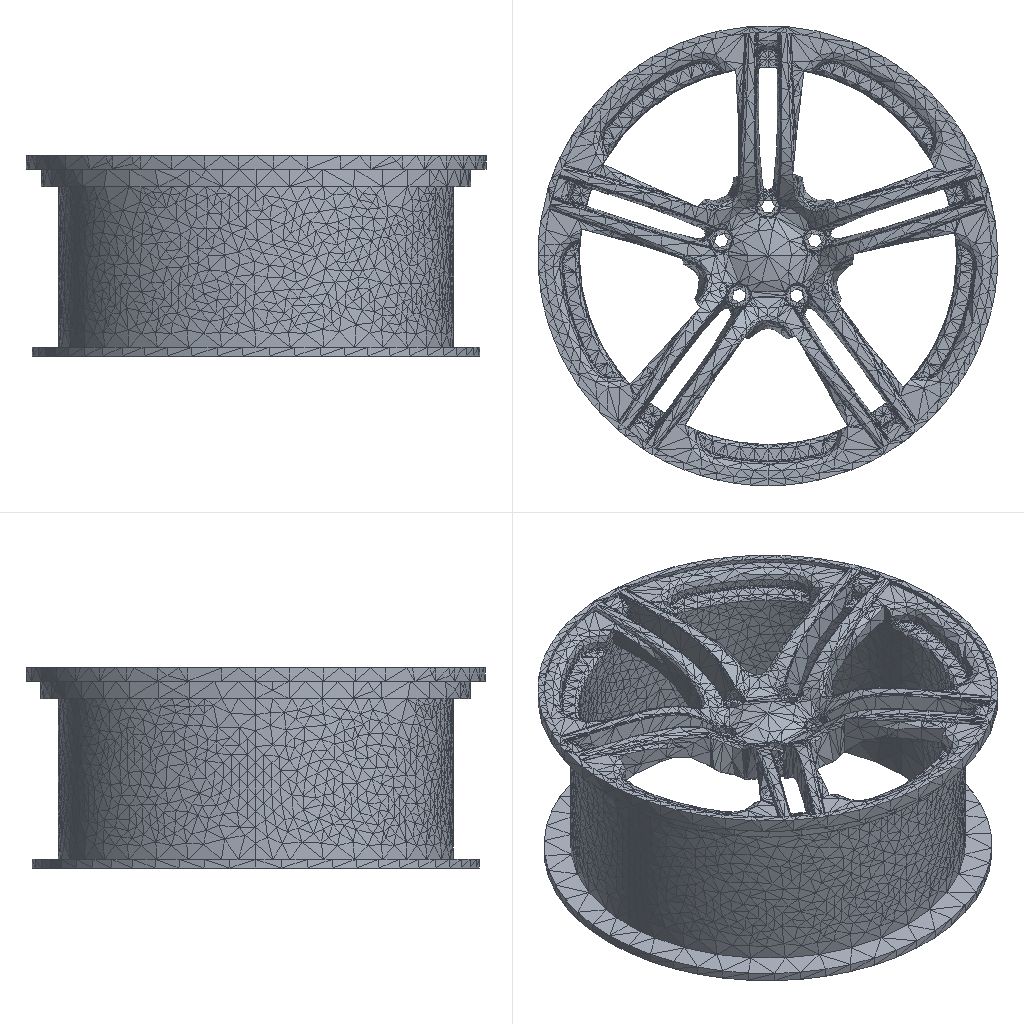Simulation study | ansys workbench
Set-up summary:
category,name,step,type,value,unit,region
solver,ansys_workbench
units,mm-N-s-tonne (MPa),,stated,"/units,MPA"
analysis,LS1,,static
load_step,LS1,LS1,static,nsubst=1; time=1
mesh,nodes,,,48309
mesh,elements,,,28563
element_type,SOLID187,,,26023
element_type,SURF154,,,2540
material,Structural Steel,,E,200000,tonne s^-2 mm^-1
material,Structural Steel,,nu,0.3
material,Structural Steel,,density,7.85e-09,tonne mm^-3
material,Structural Steel,,conductivity,60.5,tonne mm s^-3 C^-1
material,Structural Steel,,specific_heat,4.34e+08,mm^2 s^-2 C^-1
material,Structural Steel,,cte,1.2e-05,C^-1
material,Structural Steel,,permeability,10000
material,Structural Steel,,resistivity,0.00017,ohm mm
load,Define Force Using Surface Effect Elements,LS1,surface-effect pres face 2,-0.01932,,SURF154 #2
bc,Fixed Supports,model,fixed,[dofs=ALL],,_FIXEDSU
named_set,_FIXEDSU,,node,533
Ansys APDL input file, long lists of numbers shortened:
/batch
/config,noeldb,1     ! force off writing results to database
*get,_wallstrt,active,,time,wall
! ANSYS input file written by Workbench version 2022 R1
! File used for geometry attach:
/title,wbnew--____ (B5)
! ****** Begin Custom Load Command Snippet ******
/COM, ACT Extensions:
/COM,     LSDYNA, 2021.1
/COM,
! ****** End   Custom Load Command Snippet ******
*DIM,_wb_ProjectScratch_dir,string,248
_wb_ProjectScratch_dir(1) = ''
*DIM,_wb_SolverFiles_dir,string,248
_wb_SolverFiles_dir(1) = ''
*DIM,_wb_userfiles_dir,string,248
_wb_userfiles_dir(1) = ''
/com,--- Data in consistent NMM units. See Solving Units in the help system for more information.
/units,MPA
/nopr
/wb,file,start              !  signify a WB generated input file
/prep7
! Turn off shape checking because checks already performed inside WB mesher.
! See help system for more information.
SHPP,OFF,,NOWARN
/nolist
etcon,set             ! allow ANSYS to choose best KEYOP's for 180x elements, resets any applicable keyopt to MAPDL defaults
/com,*********** Nodes for the whole assembly ***********
nblock,3,,53139
(1i9,3e20.9e3)
        1     4.963852045E+01    -6.002546980E+01     4.400000000E+01
! (48308 more lines like these left out)
-1
/wb,elem,start            !  set before creation of elements
/com,*********** Elements for Body 1 "______001-FreeParts|RIM[1]" ***********
et,1,187
eblock,19,solid,,26023
(19i9)
        1        1        1        1        0        0        0        0       10        0        1     1005     1006     1497     7713    15877    15893    15878    15891
! (52045 more lines like these left out)
-1
/wb,elem,end               !  done creating elements
/com,*********** Send User Defined Coordinate System(s) ***********
csys,0
toffst,273.15,  ! Temperature offset from absolute zero
/com,*********** Set Reference Temperature ***********
tref,22.
/wb,mat,start              !  starting to send materials
/com,*********** Send Materials ***********
Temperature = 'TEMP' ! Temperature
MP,DENS,1,7.85e-09,	! tonne mm^-3
MP,ALPX,1,1.2e-05,	! C^-1
MP,C,1,434000000,	! mm^2 s^-2 C^-1
MP,KXX,1,60.5,	! tonne mm s^-3 C^-1
MP,RSVX,1,0.00017,	! ohm mm
MP,EX,1,200000,	! tonne s^-2 mm^-1
MP,NUXY,1,0.3,
MP,MURX,1,10000,
/wb,mat,end                !  done sending materials
!************************* Model Summary ********************
!______001-FreeParts|RIM[1],	结构钢,	matid,	1
!************************* End Model Summary ********************
! get the diagonal of the bounding box. Needed later for other things
*get,_xmin,node,,mnloc,x
*get,_ymin,node,,mnloc,y
*get,_zmin,node,,mnloc,z
*get,_xmax,node,,mxloc,x
*get,_ymax,node,,mxloc,y
*get,_zmax,node,,mxloc,z
_ASMDIAG=(_xmax-_xmin)*(_xmax-_xmin)+(_ymax-_ymin)*(_ymax-_ymin)+(_zmax-_zmin)*(_zmax-_zmin)
_ASMDIAG=SQRT(_ASMDIAG)
/wb,contact,start          !  starting to send contact
/wb,contact,end            !  done creating contacts
/golist
/wb,load,start             !  starting to send loads
/com,*********** Fixed Supports ***********
CMBLOCK,_FIXEDSU,NODE,      533
(8i10)
         1         9       486       487       488       491       492       493
! (66 more lines like these left out)
cmsel,s,_FIXEDSU
d,all,all
nsel,all
/com,*********** Define Force Using Surface Effect Elements ***********
local,12,0,0.,0.,0.,0.,0.,0.
csys,0
et,2,154
eblock,10,,,2540
(15i9)
    39192        2        2        2       12     2691     1341     5922     5922    18762    18771     5922    27499
! (2539 more lines like these left out)
-1
esel,s,type,,2
keyop,2,2,1                ! Apply load in local coordinate system
keyop,2,7,1                ! Use original area so load is constant in large deformation
esel,all
/gst,on,on
fini
*get,_numnode,node,0,count
*get,_numelem,elem,0,count
*get, _MAXELEMNUM, elem, 0, NUM, MAX
*get, _MAXNODENUM, node, 0, NUM, MAX
*get, _MAXELEMTYPE, etyp, 0, NUM, MAX
*get, _MAXREALCONST, real, 0, NUM, MAX
/go
/wb,load,end               !  done creating loads
/com,--- Number of total nodes = %_numnode%
/com,--- Number of contact elements = 2540
/com,--- Number of spring elements = 0
/com,--- Number of bearing elements = 0
/com,--- Number of solid elements = 26023
/com,--- Number of condensed parts = 0
/com,--- Number of total elements = %_numelem%
*get,_wallbsol,active,,time,wall
/com,****************************************************************************
/com,*************************    SOLUTION       ********************************
/com,****************************************************************************
/solu
antype,0                   ! static analysis
_thickRatio=  1     ! Ratio of thick parts in the model
eqsl,pcg,1e-8,,,,,,1
cntr,print,1               ! print out contact info and also make no initial contact an error
dmpoption,emat,no             ! Don't combine emat file for DANSYS
dmpoption,esav,no             ! Don't combine esav file for DANSYS
nldiag,cont,iter           ! print out contact info each equilibrium iteration
rescontrol,,none                 ! Do not keep any restart files
/com,****************************************************
/com,******************* SOLVE FOR LS 1 OF 1 ****************
esel,s,type,,2
nsle
sfe,all,1,pres,1,0.
sfe,all,2,pres,1,-1.93216319879701e-002
sfe,all,3,pres,1,0.
nsel,all
esel,all
/nopr
/gopr
nsub,1,1,1
time,1.
outres,erase
outres,all,none
outres,nsol,all,
outres,rsol,all
outres,eangl,all
outres,etmp,all
outres,veng,all
outres,strs,all,
outres,epel,all,
outres,eppl,all,
outres,cont,all,
! *********** WB SOLVE COMMAND ***********
! check interactive state
*get,ANSINTER_,active,,int
*if,ANSINTER_,ne,0,then
/eof
*endif
solve
/com *************** Write FE CONNECTORS *********
CEWRITE,file,ce,,INTE
/com,****************************************************
/com,*************** FINISHED SOLVE FOR LS 1 *************
*get,_wallasol,active,,time,wall
/nopr
*get,_numnode,node,0,count
*get,_numelem,elem,0,count
*get, _MAXELEMNUM, elem, 0, NUM, MAX
*get, _MAXNODENUM, node, 0, NUM, MAX,,,INTERNAL
*get, _MAXELEMTYPE, etyp, 0, NUM, MAX
*get, _MAXREALCONST, real, 0, NUM, MAX
/gopr
*get,_PCGITER,active,,solu,cgiter
/post1
xmlo,ENCODING,ISO-8859-1
xmlo,parm
/xml,parm,xml
fini
/gopr
*get,_walldone,active,,time,wall
_preptime=(_wallbsol-_wallstrt)*3600
_solvtime=(_wallasol-_wallbsol)*3600
_posttime=(_walldone-_wallasol)*3600
_totaltim=(_walldone-_wallstrt)*3600
*get,_dlbratio,active,0,solu,dlbr
*get,_combtime,active,0,solu,comb
*get,_ssmode,active,0,solu,ssmm
*get,_ndofs,active,0,solu,ndof
*get,_sol_end_time,active,0,set,time
*if,_sol_end_time,eq,1.,then
/fclean				!clean distributed files
*endif
/com,--- Total number of nodes = %_numnode%
/com,--- Total number of elements = %_numelem%
/com,--- Element load balance ratio = %_dlbratio%
/com,--- Time to combine distributed files = %_combtime%
/com,--- Sparse memory mode = %_ssmode%
/com,--- Number of DOF = %_ndofs%
/wb,file,end               ! done with WB generated input
Results summary:
result,analyses[0].index,,,1
result,analyses[0].system,,,SYS
result,analyses[0].deck,,,deck.dat
result,analyses[0].solve_status,,,completed
result,analyses[0].analysis_type,,,static
result,analyses[0].physics,,,mechanical
result,analyses[0].unit_system,,,"NMM: mm, ton, N, s, mV, mA, degC"
result,analyses[0].n_sets,,,1
result,analyses[0].load_steps[0].set,set=1,,1
result,analyses[0].load_steps[0].time_or_freq,set=1,,1
result,analyses[0].load_steps[0].max_displacement_magnitude,set=1,,0.05761
result,analyses[0].load_steps[0].max_von_mises_nodal,set=1,,16.516
result,analyses[0].load_steps[0].reaction_force_sum_xyz[1],set=1,,3.77035e-06
result,analyses[0].load_steps[0].reaction_force_sum_xyz[2],set=1,,5000
result,analyses[0].load_steps[0].reaction_force_sum_xyz[3],set=1,,-6.75443e-06